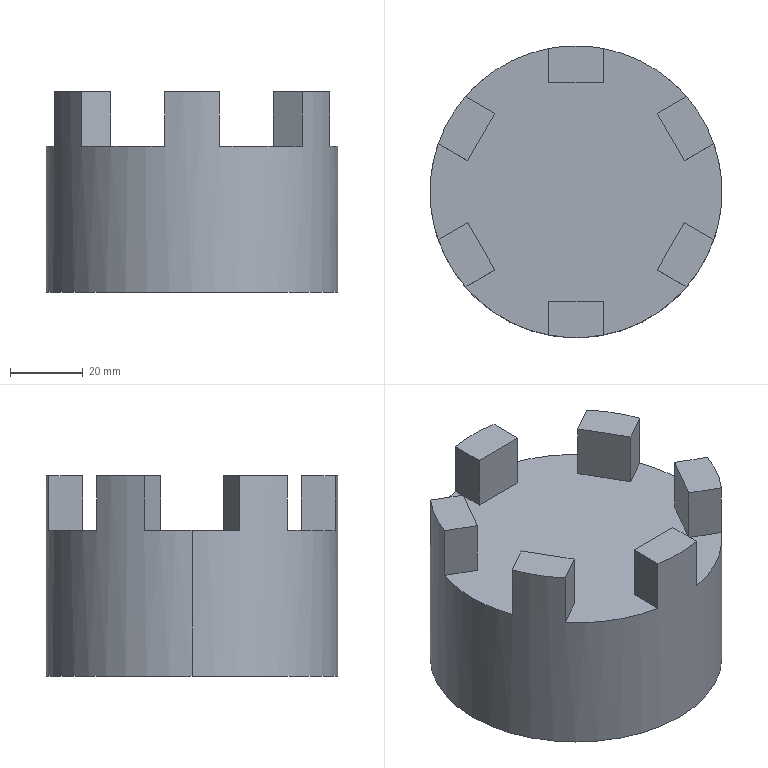Part | SolidWorks | features ICE 3, Extrusion 1 | 1 solid | 35 faces | box 80 x 80 x 55 mm | volume 187551 mm3 | plane 30 | cylinder 5 | commonest cylinder face diameters 33 x3 80 x2
STEP:
#1=CARTESIAN_POINT('',(40.,0.,40.));
#2=VERTEX_POINT('',#1);
#3=CARTESIAN_POINT('',(37.777,13.15,40.));
#4=VERTEX_POINT('',#3);
#5=CARTESIAN_POINT('',(0.,0.,40.));
#6=DIRECTION('',(0.,0.,1.));
#7=DIRECTION('',(1.,0.,0.));
#8=AXIS2_PLACEMENT_3D('',#5,#6,#7);
#9=CIRCLE('',#8,40.);
#10=EDGE_CURVE('',#2,#4,#9,.T.);
#11=ORIENTED_EDGE('',*,*,#10,.F.);
#12=CARTESIAN_POINT('',(40.,0.,0.));
#13=VERTEX_POINT('',#12);
#14=CARTESIAN_POINT('',(40.,0.,40.));
#15=DIRECTION('',(0.,0.,-1.));
#16=VECTOR('',#15,1000.);
#17=LINE('',#14,#16);
#18=EDGE_CURVE('',#2,#13,#17,.T.);
#19=ORIENTED_EDGE('',*,*,#18,.T.);
#20=CARTESIAN_POINT('',(-40.,0.,0.));
#21=VERTEX_POINT('',#20);
#22=CARTESIAN_POINT('',(0.,0.,0.));
#23=DIRECTION('',(0.,0.,1.));
#24=DIRECTION('',(1.,0.,0.));
#25=AXIS2_PLACEMENT_3D('',#22,#23,#24);
#26=CIRCLE('',#25,40.);
#27=EDGE_CURVE('',#13,#21,#26,.T.);
#28=ORIENTED_EDGE('',*,*,#27,.T.);
#29=CARTESIAN_POINT('',(-40.,0.,40.));
#30=VERTEX_POINT('',#29);
#31=CARTESIAN_POINT('',(-40.,0.,40.));
#32=DIRECTION('',(0.,0.,-1.));
#33=VECTOR('',#32,1000.);
#34=LINE('',#31,#33);
#35=EDGE_CURVE('',#30,#21,#34,.T.);
#36=ORIENTED_EDGE('',*,*,#35,.F.);
#37=CARTESIAN_POINT('',(-37.777,13.15,40.));
#38=VERTEX_POINT('',#37);
#39=CARTESIAN_POINT('',(0.,0.,40.));
#40=DIRECTION('',(0.,0.,1.));
#41=DIRECTION('',(1.,0.,0.));
#42=AXIS2_PLACEMENT_3D('',#39,#40,#41);
#43=CIRCLE('',#42,40.);
#44=EDGE_CURVE('',#38,#30,#43,.T.);
#45=ORIENTED_EDGE('',*,*,#44,.F.);
#46=CARTESIAN_POINT('',(-37.777,13.15,55.));
#47=VERTEX_POINT('',#46);
#48=CARTESIAN_POINT('',(-37.777,13.15,55.));
#49=DIRECTION('',(0.,0.,-1.));
#50=VECTOR('',#49,1000.);
#51=LINE('',#48,#50);
#52=EDGE_CURVE('',#47,#38,#51,.T.);
#53=ORIENTED_EDGE('',*,*,#52,.F.);
#54=CARTESIAN_POINT('',(-30.277,26.14,55.));
#55=VERTEX_POINT('',#54);
#56=CARTESIAN_POINT('',(0.,0.,55.));
#57=DIRECTION('',(0.,0.,1.));
#58=DIRECTION('',(1.,0.,0.));
#59=AXIS2_PLACEMENT_3D('',#56,#57,#58);
#60=CIRCLE('',#59,40.);
#61=EDGE_CURVE('',#55,#47,#60,.T.);
#62=ORIENTED_EDGE('',*,*,#61,.F.);
#63=CARTESIAN_POINT('',(-30.277,26.14,40.));
#64=VERTEX_POINT('',#63);
#65=CARTESIAN_POINT('',(-30.277,26.14,55.));
#66=DIRECTION('',(0.,0.,-1.));
#67=VECTOR('',#66,1000.);
#68=LINE('',#65,#67);
#69=EDGE_CURVE('',#55,#64,#68,.T.);
#70=ORIENTED_EDGE('',*,*,#69,.T.);
#71=CARTESIAN_POINT('',(-7.5,39.291,40.));
#72=VERTEX_POINT('',#71);
#73=CARTESIAN_POINT('',(0.,0.,40.));
#74=DIRECTION('',(0.,0.,1.));
#75=DIRECTION('',(1.,0.,0.));
#76=AXIS2_PLACEMENT_3D('',#73,#74,#75);
#77=CIRCLE('',#76,40.);
#78=EDGE_CURVE('',#72,#64,#77,.T.);
#79=ORIENTED_EDGE('',*,*,#78,.F.);
#80=CARTESIAN_POINT('',(-7.5,39.291,55.));
#81=VERTEX_POINT('',#80);
#82=CARTESIAN_POINT('',(-7.5,39.291,55.));
#83=DIRECTION('',(0.,0.,-1.));
#84=VECTOR('',#83,1000.);
#85=LINE('',#82,#84);
#86=EDGE_CURVE('',#81,#72,#85,.T.);
#87=ORIENTED_EDGE('',*,*,#86,.F.);
#88=CARTESIAN_POINT('',(7.5,39.291,55.));
#89=VERTEX_POINT('',#88);
#90=CARTESIAN_POINT('',(0.,0.,55.));
#91=DIRECTION('',(0.,0.,1.));
#92=DIRECTION('',(1.,0.,0.));
#93=AXIS2_PLACEMENT_3D('',#90,#91,#92);
#94=CIRCLE('',#93,40.);
#95=EDGE_CURVE('',#89,#81,#94,.T.);
#96=ORIENTED_EDGE('',*,*,#95,.F.);
#97=CARTESIAN_POINT('',(7.5,39.291,40.));
#98=VERTEX_POINT('',#97);
#99=CARTESIAN_POINT('',(7.5,39.291,55.));
#100=DIRECTION('',(0.,0.,-1.));
#101=VECTOR('',#100,1000.);
#102=LINE('',#99,#101);
#103=EDGE_CURVE('',#89,#98,#102,.T.);
#104=ORIENTED_EDGE('',*,*,#103,.T.);
#105=CARTESIAN_POINT('',(30.277,26.14,40.));
#106=VERTEX_POINT('',#105);
#107=CARTESIAN_POINT('',(0.,0.,40.));
#108=DIRECTION('',(0.,0.,1.));
#109=DIRECTION('',(1.,0.,0.));
#110=AXIS2_PLACEMENT_3D('',#107,#108,#109);
#111=CIRCLE('',#110,40.);
#112=EDGE_CURVE('',#106,#98,#111,.T.);
#113=ORIENTED_EDGE('',*,*,#112,.F.);
#114=CARTESIAN_POINT('',(30.277,26.14,55.));
#115=VERTEX_POINT('',#114);
#116=CARTESIAN_POINT('',(30.277,26.14,55.));
#117=DIRECTION('',(0.,0.,-1.));
#118=VECTOR('',#117,1000.);
#119=LINE('',#116,#118);
#120=EDGE_CURVE('',#115,#106,#119,.T.);
#121=ORIENTED_EDGE('',*,*,#120,.F.);
#122=CARTESIAN_POINT('',(37.777,13.15,55.));
#123=VERTEX_POINT('',#122);
#124=CARTESIAN_POINT('',(0.,0.,55.));
#125=DIRECTION('',(0.,0.,1.));
#126=DIRECTION('',(1.,0.,0.));
#127=AXIS2_PLACEMENT_3D('',#124,#125,#126);
#128=CIRCLE('',#127,40.);
#129=EDGE_CURVE('',#123,#115,#128,.T.);
#130=ORIENTED_EDGE('',*,*,#129,.F.);
#131=CARTESIAN_POINT('',(37.777,13.15,55.));
#132=DIRECTION('',(0.,0.,-1.));
#133=VECTOR('',#132,1000.);
#134=LINE('',#131,#133);
#135=EDGE_CURVE('',#123,#4,#134,.T.);
#136=ORIENTED_EDGE('',*,*,#135,.T.);
#137=EDGE_LOOP('',(#11,#19,#28,#36,#45,#53,#62,#70,#79,#87,#96,#104,#113,#121,#130,#136));
#138=FACE_OUTER_BOUND('',#137,.T.);
#139=CARTESIAN_POINT('',(0.,0.,40.));
#140=DIRECTION('',(0.,0.,-1.));
#141=DIRECTION('',(-1.,0.,0.));
#142=AXIS2_PLACEMENT_3D('',#139,#140,#141);
#143=CYLINDRICAL_SURFACE('',#142,40.);
#144=ADVANCED_FACE('',(#138),#143,.T.);
#145=CARTESIAN_POINT('',(-16.5,0.,30.));
#146=VERTEX_POINT('',#145);
#147=CARTESIAN_POINT('',(16.5,0.,30.));
#148=VERTEX_POINT('',#147);
#149=CARTESIAN_POINT('',(0.,0.,30.));
#150=DIRECTION('',(0.,0.,1.));
#151=DIRECTION('',(1.,0.,0.));
#152=AXIS2_PLACEMENT_3D('',#149,#150,#151);
#153=CIRCLE('',#152,16.5);
#154=EDGE_CURVE('',#146,#148,#153,.T.);
#155=ORIENTED_EDGE('',*,*,#154,.T.);
#156=CARTESIAN_POINT('',(16.5,0.,0.));
#157=VERTEX_POINT('',#156);
#158=CARTESIAN_POINT('',(16.5,0.,30.));
#159=DIRECTION('',(0.,0.,-1.));
#160=VECTOR('',#159,1000.);
#161=LINE('',#158,#160);
#162=EDGE_CURVE('',#148,#157,#161,.T.);
#163=ORIENTED_EDGE('',*,*,#162,.T.);
#164=CARTESIAN_POINT('',(-16.5,0.,0.));
#165=VERTEX_POINT('',#164);
#166=CARTESIAN_POINT('',(0.,0.,0.));
#167=DIRECTION('',(0.,0.,1.));
#168=DIRECTION('',(1.,0.,0.));
#169=AXIS2_PLACEMENT_3D('',#166,#167,#168);
#170=CIRCLE('',#169,16.5);
#171=EDGE_CURVE('',#165,#157,#170,.T.);
#172=ORIENTED_EDGE('',*,*,#171,.F.);
#173=CARTESIAN_POINT('',(-16.5,0.,30.));
#174=DIRECTION('',(0.,0.,-1.));
#175=VECTOR('',#174,1000.);
#176=LINE('',#173,#175);
#177=EDGE_CURVE('',#146,#165,#176,.T.);
#178=ORIENTED_EDGE('',*,*,#177,.F.);
#179=EDGE_LOOP('',(#155,#163,#172,#178));
#180=FACE_OUTER_BOUND('',#179,.T.);
#181=CARTESIAN_POINT('',(0.,0.,30.));
#182=DIRECTION('',(0.,0.,-1.));
#183=DIRECTION('',(-1.,0.,0.));
#184=AXIS2_PLACEMENT_3D('',#181,#182,#183);
#185=CYLINDRICAL_SURFACE('',#184,16.5);
#186=ADVANCED_FACE('',(#180),#185,.F.);
#187=CARTESIAN_POINT('',(-6.,15.37,30.));
#188=VERTEX_POINT('',#187);
#189=CARTESIAN_POINT('',(0.,0.,30.));
#190=DIRECTION('',(0.,0.,1.));
#191=DIRECTION('',(1.,0.,0.));
#192=AXIS2_PLACEMENT_3D('',#189,#190,#191);
#193=CIRCLE('',#192,16.5);
#194=EDGE_CURVE('',#188,#146,#193,.T.);
#195=ORIENTED_EDGE('',*,*,#194,.T.);
#196=ORIENTED_EDGE('',*,*,#177,.T.);
#197=CARTESIAN_POINT('',(-6.,15.37,0.));
#198=VERTEX_POINT('',#197);
#199=CARTESIAN_POINT('',(0.,0.,0.));
#200=DIRECTION('',(0.,0.,1.));
#201=DIRECTION('',(1.,0.,0.));
#202=AXIS2_PLACEMENT_3D('',#199,#200,#201);
#203=CIRCLE('',#202,16.5);
#204=EDGE_CURVE('',#198,#165,#203,.T.);
#205=ORIENTED_EDGE('',*,*,#204,.F.);
#206=CARTESIAN_POINT('',(-6.,15.37,30.));
#207=DIRECTION('',(0.,0.,1.));
#208=VECTOR('',#207,1000.);
#209=LINE('',#206,#208);
#210=EDGE_CURVE('',#198,#188,#209,.T.);
#211=ORIENTED_EDGE('',*,*,#210,.T.);
#212=EDGE_LOOP('',(#195,#196,#205,#211));
#213=FACE_OUTER_BOUND('',#212,.T.);
#214=CARTESIAN_POINT('',(0.,0.,30.));
#215=DIRECTION('',(0.,0.,-1.));
#216=DIRECTION('',(-1.,0.,0.));
#217=AXIS2_PLACEMENT_3D('',#214,#215,#216);
#218=CYLINDRICAL_SURFACE('',#217,16.5);
#219=ADVANCED_FACE('',(#213),#218,.F.);
#220=CARTESIAN_POINT('',(0.,0.,0.));
#221=DIRECTION('',(0.,0.,1.));
#222=DIRECTION('',(1.,0.,0.));
#223=AXIS2_PLACEMENT_3D('',#220,#221,#222);
#224=CIRCLE('',#223,40.);
#225=EDGE_CURVE('',#21,#13,#224,.T.);
#226=ORIENTED_EDGE('',*,*,#225,.F.);
#227=ORIENTED_EDGE('',*,*,#27,.F.);
#228=EDGE_LOOP('',(#226,#227));
#229=FACE_OUTER_BOUND('',#228,.T.);
#230=CARTESIAN_POINT('',(-6.,19.,0.));
#231=VERTEX_POINT('',#230);
#232=CARTESIAN_POINT('',(-6.,19.,0.));
#233=DIRECTION('',(0.,-1.,0.));
#234=VECTOR('',#233,1000.);
#235=LINE('',#232,#234);
#236=EDGE_CURVE('',#231,#198,#235,.T.);
#237=ORIENTED_EDGE('',*,*,#236,.T.);
#238=ORIENTED_EDGE('',*,*,#204,.T.);
#239=ORIENTED_EDGE('',*,*,#171,.T.);
#240=CARTESIAN_POINT('',(6.,15.37,0.));
#241=VERTEX_POINT('',#240);
#242=CARTESIAN_POINT('',(0.,0.,0.));
#243=DIRECTION('',(0.,0.,1.));
#244=DIRECTION('',(1.,0.,0.));
#245=AXIS2_PLACEMENT_3D('',#242,#243,#244);
#246=CIRCLE('',#245,16.5);
#247=EDGE_CURVE('',#157,#241,#246,.T.);
#248=ORIENTED_EDGE('',*,*,#247,.T.);
#249=CARTESIAN_POINT('',(6.,19.,0.));
#250=VERTEX_POINT('',#249);
#251=CARTESIAN_POINT('',(6.,19.,0.));
#252=DIRECTION('',(0.,-1.,0.));
#253=VECTOR('',#252,1000.);
#254=LINE('',#251,#253);
#255=EDGE_CURVE('',#250,#241,#254,.T.);
#256=ORIENTED_EDGE('',*,*,#255,.F.);
#257=CARTESIAN_POINT('',(6.,19.,0.));
#258=DIRECTION('',(-1.,0.,0.));
#259=VECTOR('',#258,1000.);
#260=LINE('',#257,#259);
#261=EDGE_CURVE('',#250,#231,#260,.T.);
#262=ORIENTED_EDGE('',*,*,#261,.T.);
#263=EDGE_LOOP('',(#237,#238,#239,#248,#256,#262));
#264=FACE_BOUND('',#263,.T.);
#265=CARTESIAN_POINT('',(0.,0.,0.));
#266=DIRECTION('',(0.,0.,1.));
#267=DIRECTION('',(1.,0.,0.));
#268=AXIS2_PLACEMENT_3D('',#265,#266,#267);
#269=PLANE('',#268);
#270=ADVANCED_FACE('',(#229,#264),#269,.F.);
#271=ORIENTED_EDGE('',*,*,#162,.F.);
#272=CARTESIAN_POINT('',(6.,15.37,30.));
#273=VERTEX_POINT('',#272);
#274=CARTESIAN_POINT('',(0.,0.,30.));
#275=DIRECTION('',(0.,0.,1.));
#276=DIRECTION('',(1.,0.,0.));
#277=AXIS2_PLACEMENT_3D('',#274,#275,#276);
#278=CIRCLE('',#277,16.5);
#279=EDGE_CURVE('',#148,#273,#278,.T.);
#280=ORIENTED_EDGE('',*,*,#279,.T.);
#281=CARTESIAN_POINT('',(6.,15.37,30.));
#282=DIRECTION('',(0.,0.,1.));
#283=VECTOR('',#282,1000.);
#284=LINE('',#281,#283);
#285=EDGE_CURVE('',#241,#273,#284,.T.);
#286=ORIENTED_EDGE('',*,*,#285,.F.);
#287=ORIENTED_EDGE('',*,*,#247,.F.);
#288=EDGE_LOOP('',(#271,#280,#286,#287));
#289=FACE_OUTER_BOUND('',#288,.T.);
#290=CARTESIAN_POINT('',(0.,0.,30.));
#291=DIRECTION('',(0.,0.,-1.));
#292=DIRECTION('',(-1.,0.,0.));
#293=AXIS2_PLACEMENT_3D('',#290,#291,#292);
#294=CYLINDRICAL_SURFACE('',#293,16.5);
#295=ADVANCED_FACE('',(#289),#294,.F.);
#296=ORIENTED_EDGE('',*,*,#18,.F.);
#297=CARTESIAN_POINT('',(37.777,-13.15,40.));
#298=VERTEX_POINT('',#297);
#299=CARTESIAN_POINT('',(0.,0.,40.));
#300=DIRECTION('',(0.,0.,1.));
#301=DIRECTION('',(1.,0.,0.));
#302=AXIS2_PLACEMENT_3D('',#299,#300,#301);
#303=CIRCLE('',#302,40.);
#304=EDGE_CURVE('',#298,#2,#303,.T.);
#305=ORIENTED_EDGE('',*,*,#304,.F.);
#306=CARTESIAN_POINT('',(37.777,-13.15,55.));
#307=VERTEX_POINT('',#306);
#308=CARTESIAN_POINT('',(37.777,-13.15,55.));
#309=DIRECTION('',(0.,0.,-1.));
#310=VECTOR('',#309,1000.);
#311=LINE('',#308,#310);
#312=EDGE_CURVE('',#307,#298,#311,.T.);
#313=ORIENTED_EDGE('',*,*,#312,.F.);
#314=CARTESIAN_POINT('',(30.277,-26.14,55.));
#315=VERTEX_POINT('',#314);
#316=CARTESIAN_POINT('',(0.,0.,55.));
#317=DIRECTION('',(0.,0.,1.));
#318=DIRECTION('',(1.,0.,0.));
#319=AXIS2_PLACEMENT_3D('',#316,#317,#318);
#320=CIRCLE('',#319,40.);
#321=EDGE_CURVE('',#315,#307,#320,.T.);
#322=ORIENTED_EDGE('',*,*,#321,.F.);
#323=CARTESIAN_POINT('',(30.277,-26.14,40.));
#324=VERTEX_POINT('',#323);
#325=CARTESIAN_POINT('',(30.277,-26.14,55.));
#326=DIRECTION('',(0.,0.,-1.));
#327=VECTOR('',#326,1000.);
#328=LINE('',#325,#327);
#329=EDGE_CURVE('',#315,#324,#328,.T.);
#330=ORIENTED_EDGE('',*,*,#329,.T.);
#331=CARTESIAN_POINT('',(7.5,-39.291,40.));
#332=VERTEX_POINT('',#331);
#333=CARTESIAN_POINT('',(0.,0.,40.));
#334=DIRECTION('',(0.,0.,1.));
#335=DIRECTION('',(1.,0.,0.));
#336=AXIS2_PLACEMENT_3D('',#333,#334,#335);
#337=CIRCLE('',#336,40.);
#338=EDGE_CURVE('',#332,#324,#337,.T.);
#339=ORIENTED_EDGE('',*,*,#338,.F.);
#340=CARTESIAN_POINT('',(7.5,-39.291,55.));
#341=VERTEX_POINT('',#340);
#342=CARTESIAN_POINT('',(7.5,-39.291,55.));
#343=DIRECTION('',(0.,0.,-1.));
#344=VECTOR('',#343,1000.);
#345=LINE('',#342,#344);
#346=EDGE_CURVE('',#341,#332,#345,.T.);
#347=ORIENTED_EDGE('',*,*,#346,.F.);
#348=CARTESIAN_POINT('',(-7.5,-39.291,55.));
#349=VERTEX_POINT('',#348);
#350=CARTESIAN_POINT('',(0.,0.,55.));
#351=DIRECTION('',(0.,0.,1.));
#352=DIRECTION('',(1.,0.,0.));
#353=AXIS2_PLACEMENT_3D('',#350,#351,#352);
#354=CIRCLE('',#353,40.);
#355=EDGE_CURVE('',#349,#341,#354,.T.);
#356=ORIENTED_EDGE('',*,*,#355,.F.);
#357=CARTESIAN_POINT('',(-7.5,-39.291,40.));
#358=VERTEX_POINT('',#357);
#359=CARTESIAN_POINT('',(-7.5,-39.291,55.));
#360=DIRECTION('',(0.,0.,-1.));
#361=VECTOR('',#360,1000.);
#362=LINE('',#359,#361);
#363=EDGE_CURVE('',#349,#358,#362,.T.);
#364=ORIENTED_EDGE('',*,*,#363,.T.);
#365=CARTESIAN_POINT('',(-30.277,-26.14,40.));
#366=VERTEX_POINT('',#365);
#367=CARTESIAN_POINT('',(0.,0.,40.));
#368=DIRECTION('',(0.,0.,1.));
#369=DIRECTION('',(1.,0.,0.));
#370=AXIS2_PLACEMENT_3D('',#367,#368,#369);
#371=CIRCLE('',#370,40.);
#372=EDGE_CURVE('',#366,#358,#371,.T.);
#373=ORIENTED_EDGE('',*,*,#372,.F.);
#374=CARTESIAN_POINT('',(-30.277,-26.14,55.));
#375=VERTEX_POINT('',#374);
#376=CARTESIAN_POINT('',(-30.277,-26.14,55.));
#377=DIRECTION('',(0.,0.,-1.));
#378=VECTOR('',#377,1000.);
#379=LINE('',#376,#378);
#380=EDGE_CURVE('',#375,#366,#379,.T.);
#381=ORIENTED_EDGE('',*,*,#380,.F.);
#382=CARTESIAN_POINT('',(-37.777,-13.15,55.));
#383=VERTEX_POINT('',#382);
#384=CARTESIAN_POINT('',(0.,0.,55.));
#385=DIRECTION('',(0.,0.,1.));
#386=DIRECTION('',(1.,0.,0.));
#387=AXIS2_PLACEMENT_3D('',#384,#385,#386);
#388=CIRCLE('',#387,40.);
#389=EDGE_CURVE('',#383,#375,#388,.T.);
#390=ORIENTED_EDGE('',*,*,#389,.F.);
#391=CARTESIAN_POINT('',(-37.777,-13.15,40.));
#392=VERTEX_POINT('',#391);
#393=CARTESIAN_POINT('',(-37.777,-13.15,55.));
#394=DIRECTION('',(0.,0.,-1.));
#395=VECTOR('',#394,1000.);
#396=LINE('',#393,#395);
#397=EDGE_CURVE('',#383,#392,#396,.T.);
#398=ORIENTED_EDGE('',*,*,#397,.T.);
#399=CARTESIAN_POINT('',(0.,0.,40.));
#400=DIRECTION('',(0.,0.,1.));
#401=DIRECTION('',(1.,0.,0.));
#402=AXIS2_PLACEMENT_3D('',#399,#400,#401);
#403=CIRCLE('',#402,40.);
#404=EDGE_CURVE('',#30,#392,#403,.T.);
#405=ORIENTED_EDGE('',*,*,#404,.F.);
#406=ORIENTED_EDGE('',*,*,#35,.T.);
#407=ORIENTED_EDGE('',*,*,#225,.T.);
#408=EDGE_LOOP('',(#296,#305,#313,#322,#330,#339,#347,#356,#364,#373,#381,#390,#398,#405,#406,#407));
#409=FACE_OUTER_BOUND('',#408,.T.);
#410=CARTESIAN_POINT('',(0.,0.,40.));
#411=DIRECTION('',(0.,0.,-1.));
#412=DIRECTION('',(-1.,0.,0.));
#413=AXIS2_PLACEMENT_3D('',#410,#411,#412);
#414=CYLINDRICAL_SURFACE('',#413,40.);
#415=ADVANCED_FACE('',(#409),#414,.T.);
#416=CARTESIAN_POINT('',(7.5,30.,40.));
#417=VERTEX_POINT('',#416);
#418=CARTESIAN_POINT('',(7.5,39.291,40.));
#419=DIRECTION('',(0.,1.,0.));
#420=VECTOR('',#419,1000.);
#421=LINE('',#418,#420);
#422=EDGE_CURVE('',#417,#98,#421,.T.);
#423=ORIENTED_EDGE('',*,*,#422,.F.);
#424=CARTESIAN_POINT('',(-7.5,30.,40.));
#425=VERTEX_POINT('',#424);
#426=CARTESIAN_POINT('',(-7.5,30.,40.));
#427=DIRECTION('',(1.,0.,0.));
#428=VECTOR('',#427,1000.);
#429=LINE('',#426,#428);
#430=EDGE_CURVE('',#425,#417,#429,.T.);
#431=ORIENTED_EDGE('',*,*,#430,.F.);
#432=CARTESIAN_POINT('',(-7.5,39.291,40.));
#433=DIRECTION('',(0.,-1.,0.));
#434=VECTOR('',#433,1000.);
#435=LINE('',#432,#434);
#436=EDGE_CURVE('',#72,#425,#435,.T.);
#437=ORIENTED_EDGE('',*,*,#436,.F.);
#438=ORIENTED_EDGE('',*,*,#78,.T.);
#439=CARTESIAN_POINT('',(-22.231,21.495,40.));
#440=VERTEX_POINT('',#439);
#441=CARTESIAN_POINT('',(-30.277,26.14,40.));
#442=DIRECTION('',(-0.866,0.5,0.));
#443=VECTOR('',#442,1000.);
#444=LINE('',#441,#443);
#445=EDGE_CURVE('',#440,#64,#444,.T.);
#446=ORIENTED_EDGE('',*,*,#445,.F.);
#447=CARTESIAN_POINT('',(-29.731,8.505,40.));
#448=VERTEX_POINT('',#447);
#449=CARTESIAN_POINT('',(-29.731,8.505,40.));
#450=DIRECTION('',(0.5,0.866,0.));
#451=VECTOR('',#450,1000.);
#452=LINE('',#449,#451);
#453=EDGE_CURVE('',#448,#440,#452,.T.);
#454=ORIENTED_EDGE('',*,*,#453,.F.);
#455=CARTESIAN_POINT('',(-37.777,13.15,40.));
#456=DIRECTION('',(0.866,-0.5,0.));
#457=VECTOR('',#456,1000.);
#458=LINE('',#455,#457);
#459=EDGE_CURVE('',#38,#448,#458,.T.);
#460=ORIENTED_EDGE('',*,*,#459,.F.);
#461=ORIENTED_EDGE('',*,*,#44,.T.);
#462=ORIENTED_EDGE('',*,*,#404,.T.);
#463=CARTESIAN_POINT('',(-29.731,-8.505,40.));
#464=VERTEX_POINT('',#463);
#465=CARTESIAN_POINT('',(-37.777,-13.15,40.));
#466=DIRECTION('',(-0.866,-0.5,0.));
#467=VECTOR('',#466,1000.);
#468=LINE('',#465,#467);
#469=EDGE_CURVE('',#464,#392,#468,.T.);
#470=ORIENTED_EDGE('',*,*,#469,.F.);
#471=CARTESIAN_POINT('',(-22.231,-21.495,40.));
#472=VERTEX_POINT('',#471);
#473=CARTESIAN_POINT('',(-22.231,-21.495,40.));
#474=DIRECTION('',(-0.5,0.866,0.));
#475=VECTOR('',#474,1000.);
#476=LINE('',#473,#475);
#477=EDGE_CURVE('',#472,#464,#476,.T.);
#478=ORIENTED_EDGE('',*,*,#477,.F.);
#479=CARTESIAN_POINT('',(-30.277,-26.14,40.));
#480=DIRECTION('',(0.866,0.5,0.));
#481=VECTOR('',#480,1000.);
#482=LINE('',#479,#481);
#483=EDGE_CURVE('',#366,#472,#482,.T.);
#484=ORIENTED_EDGE('',*,*,#483,.F.);
#485=ORIENTED_EDGE('',*,*,#372,.T.);
#486=CARTESIAN_POINT('',(-7.5,-30.,40.));
#487=VERTEX_POINT('',#486);
#488=CARTESIAN_POINT('',(-7.5,-39.291,40.));
#489=DIRECTION('',(0.,-1.,0.));
#490=VECTOR('',#489,1000.);
#491=LINE('',#488,#490);
#492=EDGE_CURVE('',#487,#358,#491,.T.);
#493=ORIENTED_EDGE('',*,*,#492,.F.);
#494=CARTESIAN_POINT('',(7.5,-30.,40.));
#495=VERTEX_POINT('',#494);
#496=CARTESIAN_POINT('',(7.5,-30.,40.));
#497=DIRECTION('',(-1.,0.,0.));
#498=VECTOR('',#497,1000.);
#499=LINE('',#496,#498);
#500=EDGE_CURVE('',#495,#487,#499,.T.);
#501=ORIENTED_EDGE('',*,*,#500,.F.);
#502=CARTESIAN_POINT('',(7.5,-39.291,40.));
#503=DIRECTION('',(0.,1.,0.));
#504=VECTOR('',#503,1000.);
#505=LINE('',#502,#504);
#506=EDGE_CURVE('',#332,#495,#505,.T.);
#507=ORIENTED_EDGE('',*,*,#506,.F.);
#508=ORIENTED_EDGE('',*,*,#338,.T.);
#509=CARTESIAN_POINT('',(22.231,-21.495,40.));
#510=VERTEX_POINT('',#509);
#511=CARTESIAN_POINT('',(30.277,-26.14,40.));
#512=DIRECTION('',(0.866,-0.5,0.));
#513=VECTOR('',#512,1000.);
#514=LINE('',#511,#513);
#515=EDGE_CURVE('',#510,#324,#514,.T.);
#516=ORIENTED_EDGE('',*,*,#515,.F.);
#517=CARTESIAN_POINT('',(29.731,-8.505,40.));
#518=VERTEX_POINT('',#517);
#519=CARTESIAN_POINT('',(29.731,-8.505,40.));
#520=DIRECTION('',(-0.5,-0.866,0.));
#521=VECTOR('',#520,1000.);
#522=LINE('',#519,#521);
#523=EDGE_CURVE('',#518,#510,#522,.T.);
#524=ORIENTED_EDGE('',*,*,#523,.F.);
#525=CARTESIAN_POINT('',(37.777,-13.15,40.));
#526=DIRECTION('',(-0.866,0.5,0.));
#527=VECTOR('',#526,1000.);
#528=LINE('',#525,#527);
#529=EDGE_CURVE('',#298,#518,#528,.T.);
#530=ORIENTED_EDGE('',*,*,#529,.F.);
#531=ORIENTED_EDGE('',*,*,#304,.T.);
#532=ORIENTED_EDGE('',*,*,#10,.T.);
#533=CARTESIAN_POINT('',(29.731,8.505,40.));
#534=VERTEX_POINT('',#533);
#535=CARTESIAN_POINT('',(37.777,13.15,40.));
#536=DIRECTION('',(0.866,0.5,0.));
#537=VECTOR('',#536,1000.);
#538=LINE('',#535,#537);
#539=EDGE_CURVE('',#534,#4,#538,.T.);
#540=ORIENTED_EDGE('',*,*,#539,.F.);
#541=CARTESIAN_POINT('',(22.231,21.495,40.));
#542=VERTEX_POINT('',#541);
#543=CARTESIAN_POINT('',(22.231,21.495,40.));
#544=DIRECTION('',(0.5,-0.866,0.));
#545=VECTOR('',#544,1000.);
#546=LINE('',#543,#545);
#547=EDGE_CURVE('',#542,#534,#546,.T.);
#548=ORIENTED_EDGE('',*,*,#547,.F.);
#549=CARTESIAN_POINT('',(30.277,26.14,40.));
#550=DIRECTION('',(-0.866,-0.5,0.));
#551=VECTOR('',#550,1000.);
#552=LINE('',#549,#551);
#553=EDGE_CURVE('',#106,#542,#552,.T.);
#554=ORIENTED_EDGE('',*,*,#553,.F.);
#555=ORIENTED_EDGE('',*,*,#112,.T.);
#556=EDGE_LOOP('',(#423,#431,#437,#438,#446,#454,#460,#461,#462,#470,#478,#484,#485,#493,#501,#507,#508,#516,#524,#530,#531,#532,#540,#548,#554,#555));
#557=FACE_OUTER_BOUND('',#556,.T.);
#558=CARTESIAN_POINT('',(0.,0.,40.));
#559=DIRECTION('',(0.,0.,1.));
#560=DIRECTION('',(1.,0.,0.));
#561=AXIS2_PLACEMENT_3D('',#558,#559,#560);
#562=PLANE('',#561);
#563=ADVANCED_FACE('',(#557),#562,.T.);
#564=ORIENTED_EDGE('',*,*,#194,.F.);
#565=CARTESIAN_POINT('',(-6.,19.,30.));
#566=VERTEX_POINT('',#565);
#567=CARTESIAN_POINT('',(-6.,19.,30.));
#568=DIRECTION('',(0.,-1.,0.));
#569=VECTOR('',#568,1000.);
#570=LINE('',#567,#569);
#571=EDGE_CURVE('',#566,#188,#570,.T.);
#572=ORIENTED_EDGE('',*,*,#571,.F.);
#573=CARTESIAN_POINT('',(6.,19.,30.));
#574=VERTEX_POINT('',#573);
#575=CARTESIAN_POINT('',(6.,19.,30.));
#576=DIRECTION('',(-1.,0.,0.));
#577=VECTOR('',#576,1000.);
#578=LINE('',#575,#577);
#579=EDGE_CURVE('',#574,#566,#578,.T.);
#580=ORIENTED_EDGE('',*,*,#579,.F.);
#581=CARTESIAN_POINT('',(6.,19.,30.));
#582=DIRECTION('',(0.,-1.,0.));
#583=VECTOR('',#582,1000.);
#584=LINE('',#581,#583);
#585=EDGE_CURVE('',#574,#273,#584,.T.);
#586=ORIENTED_EDGE('',*,*,#585,.T.);
#587=ORIENTED_EDGE('',*,*,#279,.F.);
#588=ORIENTED_EDGE('',*,*,#154,.F.);
#589=EDGE_LOOP('',(#564,#572,#580,#586,#587,#588));
#590=FACE_OUTER_BOUND('',#589,.T.);
#591=CARTESIAN_POINT('',(0.,0.,30.));
#592=DIRECTION('',(0.,0.,1.));
#593=DIRECTION('',(1.,0.,0.));
#594=AXIS2_PLACEMENT_3D('',#591,#592,#593);
#595=PLANE('',#594);
#596=ADVANCED_FACE('',(#590),#595,.F.);
#597=ORIENTED_EDGE('',*,*,#539,.T.);
#598=ORIENTED_EDGE('',*,*,#135,.F.);
#599=CARTESIAN_POINT('',(29.731,8.505,55.));
#600=VERTEX_POINT('',#599);
#601=CARTESIAN_POINT('',(37.777,13.15,55.));
#602=DIRECTION('',(0.866,0.5,0.));
#603=VECTOR('',#602,1000.);
#604=LINE('',#601,#603);
#605=EDGE_CURVE('',#600,#123,#604,.T.);
#606=ORIENTED_EDGE('',*,*,#605,.F.);
#607=CARTESIAN_POINT('',(29.731,8.505,55.));
#608=DIRECTION('',(0.,0.,-1.));
#609=VECTOR('',#608,1000.);
#610=LINE('',#607,#609);
#611=EDGE_CURVE('',#600,#534,#610,.T.);
#612=ORIENTED_EDGE('',*,*,#611,.T.);
#613=EDGE_LOOP('',(#597,#598,#606,#612));
#614=FACE_OUTER_BOUND('',#613,.T.);
#615=CARTESIAN_POINT('',(37.777,13.15,55.));
#616=DIRECTION('',(-0.5,0.866,0.));
#617=DIRECTION('',(-0.866,-0.5,0.));
#618=AXIS2_PLACEMENT_3D('',#615,#616,#617);
#619=PLANE('',#618);
#620=ADVANCED_FACE('',(#614),#619,.F.);
#621=ORIENTED_EDGE('',*,*,#553,.T.);
#622=CARTESIAN_POINT('',(22.231,21.495,55.));
#623=VERTEX_POINT('',#622);
#624=CARTESIAN_POINT('',(22.231,21.495,55.));
#625=DIRECTION('',(0.,0.,-1.));
#626=VECTOR('',#625,1000.);
#627=LINE('',#624,#626);
#628=EDGE_CURVE('',#623,#542,#627,.T.);
#629=ORIENTED_EDGE('',*,*,#628,.F.);
#630=CARTESIAN_POINT('',(30.277,26.14,55.));
#631=DIRECTION('',(-0.866,-0.5,0.));
#632=VECTOR('',#631,1000.);
#633=LINE('',#630,#632);
#634=EDGE_CURVE('',#115,#623,#633,.T.);
#635=ORIENTED_EDGE('',*,*,#634,.F.);
#636=ORIENTED_EDGE('',*,*,#120,.T.);
#637=EDGE_LOOP('',(#621,#629,#635,#636));
#638=FACE_OUTER_BOUND('',#637,.T.);
#639=CARTESIAN_POINT('',(30.277,26.14,55.));
#640=DIRECTION('',(0.5,-0.866,0.));
#641=DIRECTION('',(0.866,0.5,0.));
#642=AXIS2_PLACEMENT_3D('',#639,#640,#641);
#643=PLANE('',#642);
#644=ADVANCED_FACE('',(#638),#643,.F.);
#645=ORIENTED_EDGE('',*,*,#547,.T.);
#646=ORIENTED_EDGE('',*,*,#611,.F.);
#647=CARTESIAN_POINT('',(22.231,21.495,55.));
#648=DIRECTION('',(0.5,-0.866,0.));
#649=VECTOR('',#648,1000.);
#650=LINE('',#647,#649);
#651=EDGE_CURVE('',#623,#600,#650,.T.);
#652=ORIENTED_EDGE('',*,*,#651,.F.);
#653=ORIENTED_EDGE('',*,*,#628,.T.);
#654=EDGE_LOOP('',(#645,#646,#652,#653));
#655=FACE_OUTER_BOUND('',#654,.T.);
#656=CARTESIAN_POINT('',(22.231,21.495,55.));
#657=DIRECTION('',(0.866,0.5,0.));
#658=DIRECTION('',(-0.5,0.866,0.));
#659=AXIS2_PLACEMENT_3D('',#656,#657,#658);
#660=PLANE('',#659);
#661=ADVANCED_FACE('',(#655),#660,.F.);
#662=ORIENTED_EDGE('',*,*,#605,.T.);
#663=ORIENTED_EDGE('',*,*,#129,.T.);
#664=ORIENTED_EDGE('',*,*,#634,.T.);
#665=ORIENTED_EDGE('',*,*,#651,.T.);
#666=EDGE_LOOP('',(#662,#663,#664,#665));
#667=FACE_OUTER_BOUND('',#666,.T.);
#668=CARTESIAN_POINT('',(0.,0.,55.));
#669=DIRECTION('',(0.,0.,1.));
#670=DIRECTION('',(1.,0.,0.));
#671=AXIS2_PLACEMENT_3D('',#668,#669,#670);
#672=PLANE('',#671);
#673=ADVANCED_FACE('',(#667),#672,.T.);
#674=ORIENTED_EDGE('',*,*,#515,.T.);
#675=ORIENTED_EDGE('',*,*,#329,.F.);
#676=CARTESIAN_POINT('',(22.231,-21.495,55.));
#677=VERTEX_POINT('',#676);
#678=CARTESIAN_POINT('',(30.277,-26.14,55.));
#679=DIRECTION('',(0.866,-0.5,0.));
#680=VECTOR('',#679,1000.);
#681=LINE('',#678,#680);
#682=EDGE_CURVE('',#677,#315,#681,.T.);
#683=ORIENTED_EDGE('',*,*,#682,.F.);
#684=CARTESIAN_POINT('',(22.231,-21.495,55.));
#685=DIRECTION('',(0.,0.,-1.));
#686=VECTOR('',#685,1000.);
#687=LINE('',#684,#686);
#688=EDGE_CURVE('',#677,#510,#687,.T.);
#689=ORIENTED_EDGE('',*,*,#688,.T.);
#690=EDGE_LOOP('',(#674,#675,#683,#689));
#691=FACE_OUTER_BOUND('',#690,.T.);
#692=CARTESIAN_POINT('',(30.277,-26.14,55.));
#693=DIRECTION('',(0.5,0.866,0.));
#694=DIRECTION('',(-0.866,0.5,0.));
#695=AXIS2_PLACEMENT_3D('',#692,#693,#694);
#696=PLANE('',#695);
#697=ADVANCED_FACE('',(#691),#696,.F.);
#698=ORIENTED_EDGE('',*,*,#529,.T.);
#699=CARTESIAN_POINT('',(29.731,-8.505,55.));
#700=VERTEX_POINT('',#699);
#701=CARTESIAN_POINT('',(29.731,-8.505,55.));
#702=DIRECTION('',(0.,0.,-1.));
#703=VECTOR('',#702,1000.);
#704=LINE('',#701,#703);
#705=EDGE_CURVE('',#700,#518,#704,.T.);
#706=ORIENTED_EDGE('',*,*,#705,.F.);
#707=CARTESIAN_POINT('',(37.777,-13.15,55.));
#708=DIRECTION('',(-0.866,0.5,0.));
#709=VECTOR('',#708,1000.);
#710=LINE('',#707,#709);
#711=EDGE_CURVE('',#307,#700,#710,.T.);
#712=ORIENTED_EDGE('',*,*,#711,.F.);
#713=ORIENTED_EDGE('',*,*,#312,.T.);
#714=EDGE_LOOP('',(#698,#706,#712,#713));
#715=FACE_OUTER_BOUND('',#714,.T.);
#716=CARTESIAN_POINT('',(37.777,-13.15,55.));
#717=DIRECTION('',(-0.5,-0.866,0.));
#718=DIRECTION('',(0.866,-0.5,0.));
#719=AXIS2_PLACEMENT_3D('',#716,#717,#718);
#720=PLANE('',#719);
#721=ADVANCED_FACE('',(#715),#720,.F.);
#722=ORIENTED_EDGE('',*,*,#523,.T.);
#723=ORIENTED_EDGE('',*,*,#688,.F.);
#724=CARTESIAN_POINT('',(29.731,-8.505,55.));
#725=DIRECTION('',(-0.5,-0.866,0.));
#726=VECTOR('',#725,1000.);
#727=LINE('',#724,#726);
#728=EDGE_CURVE('',#700,#677,#727,.T.);
#729=ORIENTED_EDGE('',*,*,#728,.F.);
#730=ORIENTED_EDGE('',*,*,#705,.T.);
#731=EDGE_LOOP('',(#722,#723,#729,#730));
#732=FACE_OUTER_BOUND('',#731,.T.);
#733=CARTESIAN_POINT('',(29.731,-8.505,55.));
#734=DIRECTION('',(0.866,-0.5,0.));
#735=DIRECTION('',(0.5,0.866,0.));
#736=AXIS2_PLACEMENT_3D('',#733,#734,#735);
#737=PLANE('',#736);
#738=ADVANCED_FACE('',(#732),#737,.F.);
#739=ORIENTED_EDGE('',*,*,#682,.T.);
#740=ORIENTED_EDGE('',*,*,#321,.T.);
#741=ORIENTED_EDGE('',*,*,#711,.T.);
#742=ORIENTED_EDGE('',*,*,#728,.T.);
#743=EDGE_LOOP('',(#739,#740,#741,#742));
#744=FACE_OUTER_BOUND('',#743,.T.);
#745=CARTESIAN_POINT('',(0.,0.,55.));
#746=DIRECTION('',(0.,0.,1.));
#747=DIRECTION('',(1.,0.,0.));
#748=AXIS2_PLACEMENT_3D('',#745,#746,#747);
#749=PLANE('',#748);
#750=ADVANCED_FACE('',(#744),#749,.T.);
#751=ORIENTED_EDGE('',*,*,#492,.T.);
#752=ORIENTED_EDGE('',*,*,#363,.F.);
#753=CARTESIAN_POINT('',(-7.5,-30.,55.));
#754=VERTEX_POINT('',#753);
#755=CARTESIAN_POINT('',(-7.5,-39.291,55.));
#756=DIRECTION('',(0.,-1.,0.));
#757=VECTOR('',#756,1000.);
#758=LINE('',#755,#757);
#759=EDGE_CURVE('',#754,#349,#758,.T.);
#760=ORIENTED_EDGE('',*,*,#759,.F.);
#761=CARTESIAN_POINT('',(-7.5,-30.,55.));
#762=DIRECTION('',(0.,0.,-1.));
#763=VECTOR('',#762,1000.);
#764=LINE('',#761,#763);
#765=EDGE_CURVE('',#754,#487,#764,.T.);
#766=ORIENTED_EDGE('',*,*,#765,.T.);
#767=EDGE_LOOP('',(#751,#752,#760,#766));
#768=FACE_OUTER_BOUND('',#767,.T.);
#769=CARTESIAN_POINT('',(-7.5,-39.291,55.));
#770=DIRECTION('',(1.,0.,0.));
#771=DIRECTION('',(0.,1.,0.));
#772=AXIS2_PLACEMENT_3D('',#769,#770,#771);
#773=PLANE('',#772);
#774=ADVANCED_FACE('',(#768),#773,.F.);
#775=ORIENTED_EDGE('',*,*,#506,.T.);
#776=CARTESIAN_POINT('',(7.5,-30.,55.));
#777=VERTEX_POINT('',#776);
#778=CARTESIAN_POINT('',(7.5,-30.,55.));
#779=DIRECTION('',(0.,0.,-1.));
#780=VECTOR('',#779,1000.);
#781=LINE('',#778,#780);
#782=EDGE_CURVE('',#777,#495,#781,.T.);
#783=ORIENTED_EDGE('',*,*,#782,.F.);
#784=CARTESIAN_POINT('',(7.5,-39.291,55.));
#785=DIRECTION('',(0.,1.,0.));
#786=VECTOR('',#785,1000.);
#787=LINE('',#784,#786);
#788=EDGE_CURVE('',#341,#777,#787,.T.);
#789=ORIENTED_EDGE('',*,*,#788,.F.);
#790=ORIENTED_EDGE('',*,*,#346,.T.);
#791=EDGE_LOOP('',(#775,#783,#789,#790));
#792=FACE_OUTER_BOUND('',#791,.T.);
#793=CARTESIAN_POINT('',(7.5,-39.291,55.));
#794=DIRECTION('',(-1.,0.,0.));
#795=DIRECTION('',(0.,-1.,0.));
#796=AXIS2_PLACEMENT_3D('',#793,#794,#795);
#797=PLANE('',#796);
#798=ADVANCED_FACE('',(#792),#797,.F.);
#799=ORIENTED_EDGE('',*,*,#500,.T.);
#800=ORIENTED_EDGE('',*,*,#765,.F.);
#801=CARTESIAN_POINT('',(7.5,-30.,55.));
#802=DIRECTION('',(-1.,0.,0.));
#803=VECTOR('',#802,1000.);
#804=LINE('',#801,#803);
#805=EDGE_CURVE('',#777,#754,#804,.T.);
#806=ORIENTED_EDGE('',*,*,#805,.F.);
#807=ORIENTED_EDGE('',*,*,#782,.T.);
#808=EDGE_LOOP('',(#799,#800,#806,#807));
#809=FACE_OUTER_BOUND('',#808,.T.);
#810=CARTESIAN_POINT('',(7.5,-30.,55.));
#811=DIRECTION('',(0.,-1.,0.));
#812=DIRECTION('',(1.,0.,0.));
#813=AXIS2_PLACEMENT_3D('',#810,#811,#812);
#814=PLANE('',#813);
#815=ADVANCED_FACE('',(#809),#814,.F.);
#816=ORIENTED_EDGE('',*,*,#759,.T.);
#817=ORIENTED_EDGE('',*,*,#355,.T.);
#818=ORIENTED_EDGE('',*,*,#788,.T.);
#819=ORIENTED_EDGE('',*,*,#805,.T.);
#820=EDGE_LOOP('',(#816,#817,#818,#819));
#821=FACE_OUTER_BOUND('',#820,.T.);
#822=CARTESIAN_POINT('',(0.,0.,55.));
#823=DIRECTION('',(0.,0.,1.));
#824=DIRECTION('',(1.,0.,0.));
#825=AXIS2_PLACEMENT_3D('',#822,#823,#824);
#826=PLANE('',#825);
#827=ADVANCED_FACE('',(#821),#826,.T.);
#828=ORIENTED_EDGE('',*,*,#469,.T.);
#829=ORIENTED_EDGE('',*,*,#397,.F.);
#830=CARTESIAN_POINT('',(-29.731,-8.505,55.));
#831=VERTEX_POINT('',#830);
#832=CARTESIAN_POINT('',(-37.777,-13.15,55.));
#833=DIRECTION('',(-0.866,-0.5,0.));
#834=VECTOR('',#833,1000.);
#835=LINE('',#832,#834);
#836=EDGE_CURVE('',#831,#383,#835,.T.);
#837=ORIENTED_EDGE('',*,*,#836,.F.);
#838=CARTESIAN_POINT('',(-29.731,-8.505,55.));
#839=DIRECTION('',(0.,0.,-1.));
#840=VECTOR('',#839,1000.);
#841=LINE('',#838,#840);
#842=EDGE_CURVE('',#831,#464,#841,.T.);
#843=ORIENTED_EDGE('',*,*,#842,.T.);
#844=EDGE_LOOP('',(#828,#829,#837,#843));
#845=FACE_OUTER_BOUND('',#844,.T.);
#846=CARTESIAN_POINT('',(-37.777,-13.15,55.));
#847=DIRECTION('',(0.5,-0.866,0.));
#848=DIRECTION('',(0.866,0.5,0.));
#849=AXIS2_PLACEMENT_3D('',#846,#847,#848);
#850=PLANE('',#849);
#851=ADVANCED_FACE('',(#845),#850,.F.);
#852=ORIENTED_EDGE('',*,*,#483,.T.);
#853=CARTESIAN_POINT('',(-22.231,-21.495,55.));
#854=VERTEX_POINT('',#853);
#855=CARTESIAN_POINT('',(-22.231,-21.495,55.));
#856=DIRECTION('',(0.,0.,-1.));
#857=VECTOR('',#856,1000.);
#858=LINE('',#855,#857);
#859=EDGE_CURVE('',#854,#472,#858,.T.);
#860=ORIENTED_EDGE('',*,*,#859,.F.);
#861=CARTESIAN_POINT('',(-30.277,-26.14,55.));
#862=DIRECTION('',(0.866,0.5,0.));
#863=VECTOR('',#862,1000.);
#864=LINE('',#861,#863);
#865=EDGE_CURVE('',#375,#854,#864,.T.);
#866=ORIENTED_EDGE('',*,*,#865,.F.);
#867=ORIENTED_EDGE('',*,*,#380,.T.);
#868=EDGE_LOOP('',(#852,#860,#866,#867));
#869=FACE_OUTER_BOUND('',#868,.T.);
#870=CARTESIAN_POINT('',(-30.277,-26.14,55.));
#871=DIRECTION('',(-0.5,0.866,0.));
#872=DIRECTION('',(-0.866,-0.5,0.));
#873=AXIS2_PLACEMENT_3D('',#870,#871,#872);
#874=PLANE('',#873);
#875=ADVANCED_FACE('',(#869),#874,.F.);
#876=ORIENTED_EDGE('',*,*,#477,.T.);
#877=ORIENTED_EDGE('',*,*,#842,.F.);
#878=CARTESIAN_POINT('',(-22.231,-21.495,55.));
#879=DIRECTION('',(-0.5,0.866,0.));
#880=VECTOR('',#879,1000.);
#881=LINE('',#878,#880);
#882=EDGE_CURVE('',#854,#831,#881,.T.);
#883=ORIENTED_EDGE('',*,*,#882,.F.);
#884=ORIENTED_EDGE('',*,*,#859,.T.);
#885=EDGE_LOOP('',(#876,#877,#883,#884));
#886=FACE_OUTER_BOUND('',#885,.T.);
#887=CARTESIAN_POINT('',(-22.231,-21.495,55.));
#888=DIRECTION('',(-0.866,-0.5,0.));
#889=DIRECTION('',(0.5,-0.866,0.));
#890=AXIS2_PLACEMENT_3D('',#887,#888,#889);
#891=PLANE('',#890);
#892=ADVANCED_FACE('',(#886),#891,.F.);
#893=ORIENTED_EDGE('',*,*,#836,.T.);
#894=ORIENTED_EDGE('',*,*,#389,.T.);
#895=ORIENTED_EDGE('',*,*,#865,.T.);
#896=ORIENTED_EDGE('',*,*,#882,.T.);
#897=EDGE_LOOP('',(#893,#894,#895,#896));
#898=FACE_OUTER_BOUND('',#897,.T.);
#899=CARTESIAN_POINT('',(0.,0.,55.));
#900=DIRECTION('',(0.,0.,1.));
#901=DIRECTION('',(1.,0.,0.));
#902=AXIS2_PLACEMENT_3D('',#899,#900,#901);
#903=PLANE('',#902);
#904=ADVANCED_FACE('',(#898),#903,.T.);
#905=ORIENTED_EDGE('',*,*,#445,.T.);
#906=ORIENTED_EDGE('',*,*,#69,.F.);
#907=CARTESIAN_POINT('',(-22.231,21.495,55.));
#908=VERTEX_POINT('',#907);
#909=CARTESIAN_POINT('',(-30.277,26.14,55.));
#910=DIRECTION('',(-0.866,0.5,0.));
#911=VECTOR('',#910,1000.);
#912=LINE('',#909,#911);
#913=EDGE_CURVE('',#908,#55,#912,.T.);
#914=ORIENTED_EDGE('',*,*,#913,.F.);
#915=CARTESIAN_POINT('',(-22.231,21.495,55.));
#916=DIRECTION('',(0.,0.,-1.));
#917=VECTOR('',#916,1000.);
#918=LINE('',#915,#917);
#919=EDGE_CURVE('',#908,#440,#918,.T.);
#920=ORIENTED_EDGE('',*,*,#919,.T.);
#921=EDGE_LOOP('',(#905,#906,#914,#920));
#922=FACE_OUTER_BOUND('',#921,.T.);
#923=CARTESIAN_POINT('',(-30.277,26.14,55.));
#924=DIRECTION('',(-0.5,-0.866,0.));
#925=DIRECTION('',(0.866,-0.5,0.));
#926=AXIS2_PLACEMENT_3D('',#923,#924,#925);
#927=PLANE('',#926);
#928=ADVANCED_FACE('',(#922),#927,.F.);
#929=ORIENTED_EDGE('',*,*,#459,.T.);
#930=CARTESIAN_POINT('',(-29.731,8.505,55.));
#931=VERTEX_POINT('',#930);
#932=CARTESIAN_POINT('',(-29.731,8.505,55.));
#933=DIRECTION('',(0.,0.,-1.));
#934=VECTOR('',#933,1000.);
#935=LINE('',#932,#934);
#936=EDGE_CURVE('',#931,#448,#935,.T.);
#937=ORIENTED_EDGE('',*,*,#936,.F.);
#938=CARTESIAN_POINT('',(-37.777,13.15,55.));
#939=DIRECTION('',(0.866,-0.5,0.));
#940=VECTOR('',#939,1000.);
#941=LINE('',#938,#940);
#942=EDGE_CURVE('',#47,#931,#941,.T.);
#943=ORIENTED_EDGE('',*,*,#942,.F.);
#944=ORIENTED_EDGE('',*,*,#52,.T.);
#945=EDGE_LOOP('',(#929,#937,#943,#944));
#946=FACE_OUTER_BOUND('',#945,.T.);
#947=CARTESIAN_POINT('',(-37.777,13.15,55.));
#948=DIRECTION('',(0.5,0.866,0.));
#949=DIRECTION('',(-0.866,0.5,0.));
#950=AXIS2_PLACEMENT_3D('',#947,#948,#949);
#951=PLANE('',#950);
#952=ADVANCED_FACE('',(#946),#951,.F.);
#953=ORIENTED_EDGE('',*,*,#453,.T.);
#954=ORIENTED_EDGE('',*,*,#919,.F.);
#955=CARTESIAN_POINT('',(-29.731,8.505,55.));
#956=DIRECTION('',(0.5,0.866,0.));
#957=VECTOR('',#956,1000.);
#958=LINE('',#955,#957);
#959=EDGE_CURVE('',#931,#908,#958,.T.);
#960=ORIENTED_EDGE('',*,*,#959,.F.);
#961=ORIENTED_EDGE('',*,*,#936,.T.);
#962=EDGE_LOOP('',(#953,#954,#960,#961));
#963=FACE_OUTER_BOUND('',#962,.T.);
#964=CARTESIAN_POINT('',(-29.731,8.505,55.));
#965=DIRECTION('',(-0.866,0.5,0.));
#966=DIRECTION('',(-0.5,-0.866,0.));
#967=AXIS2_PLACEMENT_3D('',#964,#965,#966);
#968=PLANE('',#967);
#969=ADVANCED_FACE('',(#963),#968,.F.);
#970=ORIENTED_EDGE('',*,*,#913,.T.);
#971=ORIENTED_EDGE('',*,*,#61,.T.);
#972=ORIENTED_EDGE('',*,*,#942,.T.);
#973=ORIENTED_EDGE('',*,*,#959,.T.);
#974=EDGE_LOOP('',(#970,#971,#972,#973));
#975=FACE_OUTER_BOUND('',#974,.T.);
#976=CARTESIAN_POINT('',(0.,0.,55.));
#977=DIRECTION('',(0.,0.,1.));
#978=DIRECTION('',(1.,0.,0.));
#979=AXIS2_PLACEMENT_3D('',#976,#977,#978);
#980=PLANE('',#979);
#981=ADVANCED_FACE('',(#975),#980,.T.);
#982=ORIENTED_EDGE('',*,*,#422,.T.);
#983=ORIENTED_EDGE('',*,*,#103,.F.);
#984=CARTESIAN_POINT('',(7.5,30.,55.));
#985=VERTEX_POINT('',#984);
#986=CARTESIAN_POINT('',(7.5,39.291,55.));
#987=DIRECTION('',(0.,1.,0.));
#988=VECTOR('',#987,1000.);
#989=LINE('',#986,#988);
#990=EDGE_CURVE('',#985,#89,#989,.T.);
#991=ORIENTED_EDGE('',*,*,#990,.F.);
#992=CARTESIAN_POINT('',(7.5,30.,55.));
#993=DIRECTION('',(0.,0.,-1.));
#994=VECTOR('',#993,1000.);
#995=LINE('',#992,#994);
#996=EDGE_CURVE('',#985,#417,#995,.T.);
#997=ORIENTED_EDGE('',*,*,#996,.T.);
#998=EDGE_LOOP('',(#982,#983,#991,#997));
#999=FACE_OUTER_BOUND('',#998,.T.);
#1000=CARTESIAN_POINT('',(7.5,39.291,55.));
#1001=DIRECTION('',(-1.,0.,0.));
#1002=DIRECTION('',(0.,-1.,0.));
#1003=AXIS2_PLACEMENT_3D('',#1000,#1001,#1002);
#1004=PLANE('',#1003);
#1005=ADVANCED_FACE('',(#999),#1004,.F.);
#1006=ORIENTED_EDGE('',*,*,#436,.T.);
#1007=CARTESIAN_POINT('',(-7.5,30.,55.));
#1008=VERTEX_POINT('',#1007);
#1009=CARTESIAN_POINT('',(-7.5,30.,55.));
#1010=DIRECTION('',(0.,0.,-1.));
#1011=VECTOR('',#1010,1000.);
#1012=LINE('',#1009,#1011);
#1013=EDGE_CURVE('',#1008,#425,#1012,.T.);
#1014=ORIENTED_EDGE('',*,*,#1013,.F.);
#1015=CARTESIAN_POINT('',(-7.5,39.291,55.));
#1016=DIRECTION('',(0.,-1.,0.));
#1017=VECTOR('',#1016,1000.);
#1018=LINE('',#1015,#1017);
#1019=EDGE_CURVE('',#81,#1008,#1018,.T.);
#1020=ORIENTED_EDGE('',*,*,#1019,.F.);
#1021=ORIENTED_EDGE('',*,*,#86,.T.);
#1022=EDGE_LOOP('',(#1006,#1014,#1020,#1021));
#1023=FACE_OUTER_BOUND('',#1022,.T.);
#1024=CARTESIAN_POINT('',(-7.5,39.291,55.));
#1025=DIRECTION('',(1.,0.,0.));
#1026=DIRECTION('',(0.,1.,0.));
#1027=AXIS2_PLACEMENT_3D('',#1024,#1025,#1026);
#1028=PLANE('',#1027);
#1029=ADVANCED_FACE('',(#1023),#1028,.F.);
#1030=ORIENTED_EDGE('',*,*,#430,.T.);
#1031=ORIENTED_EDGE('',*,*,#996,.F.);
#1032=CARTESIAN_POINT('',(-7.5,30.,55.));
#1033=DIRECTION('',(1.,0.,0.));
#1034=VECTOR('',#1033,1000.);
#1035=LINE('',#1032,#1034);
#1036=EDGE_CURVE('',#1008,#985,#1035,.T.);
#1037=ORIENTED_EDGE('',*,*,#1036,.F.);
#1038=ORIENTED_EDGE('',*,*,#1013,.T.);
#1039=EDGE_LOOP('',(#1030,#1031,#1037,#1038));
#1040=FACE_OUTER_BOUND('',#1039,.T.);
#1041=CARTESIAN_POINT('',(-7.5,30.,55.));
#1042=DIRECTION('',(0.,1.,0.));
#1043=DIRECTION('',(0.,0.,1.));
#1044=AXIS2_PLACEMENT_3D('',#1041,#1042,#1043);
#1045=PLANE('',#1044);
#1046=ADVANCED_FACE('',(#1040),#1045,.F.);
#1047=ORIENTED_EDGE('',*,*,#990,.T.);
#1048=ORIENTED_EDGE('',*,*,#95,.T.);
#1049=ORIENTED_EDGE('',*,*,#1019,.T.);
#1050=ORIENTED_EDGE('',*,*,#1036,.T.);
#1051=EDGE_LOOP('',(#1047,#1048,#1049,#1050));
#1052=FACE_OUTER_BOUND('',#1051,.T.);
#1053=CARTESIAN_POINT('',(0.,0.,55.));
#1054=DIRECTION('',(0.,0.,1.));
#1055=DIRECTION('',(1.,0.,0.));
#1056=AXIS2_PLACEMENT_3D('',#1053,#1054,#1055);
#1057=PLANE('',#1056);
#1058=ADVANCED_FACE('',(#1052),#1057,.T.);
#1059=ORIENTED_EDGE('',*,*,#261,.F.);
#1060=CARTESIAN_POINT('',(6.,19.,30.));
#1061=DIRECTION('',(0.,0.,-1.));
#1062=VECTOR('',#1061,1000.);
#1063=LINE('',#1060,#1062);
#1064=EDGE_CURVE('',#574,#250,#1063,.T.);
#1065=ORIENTED_EDGE('',*,*,#1064,.F.);
#1066=ORIENTED_EDGE('',*,*,#579,.T.);
#1067=CARTESIAN_POINT('',(-6.,19.,30.));
#1068=DIRECTION('',(0.,0.,-1.));
#1069=VECTOR('',#1068,1000.);
#1070=LINE('',#1067,#1069);
#1071=EDGE_CURVE('',#566,#231,#1070,.T.);
#1072=ORIENTED_EDGE('',*,*,#1071,.T.);
#1073=EDGE_LOOP('',(#1059,#1065,#1066,#1072));
#1074=FACE_OUTER_BOUND('',#1073,.T.);
#1075=CARTESIAN_POINT('',(6.,19.,30.));
#1076=DIRECTION('',(0.,-1.,0.));
#1077=DIRECTION('',(0.,0.,-1.));
#1078=AXIS2_PLACEMENT_3D('',#1075,#1076,#1077);
#1079=PLANE('',#1078);
#1080=ADVANCED_FACE('',(#1074),#1079,.T.);
#1081=ORIENTED_EDGE('',*,*,#236,.F.);
#1082=ORIENTED_EDGE('',*,*,#1071,.F.);
#1083=ORIENTED_EDGE('',*,*,#571,.T.);
#1084=ORIENTED_EDGE('',*,*,#210,.F.);
#1085=EDGE_LOOP('',(#1081,#1082,#1083,#1084));
#1086=FACE_OUTER_BOUND('',#1085,.T.);
#1087=CARTESIAN_POINT('',(-6.,19.,30.));
#1088=DIRECTION('',(1.,0.,0.));
#1089=DIRECTION('',(0.,1.,0.));
#1090=AXIS2_PLACEMENT_3D('',#1087,#1088,#1089);
#1091=PLANE('',#1090);
#1092=ADVANCED_FACE('',(#1086),#1091,.T.);
#1093=ORIENTED_EDGE('',*,*,#285,.T.);
#1094=ORIENTED_EDGE('',*,*,#585,.F.);
#1095=ORIENTED_EDGE('',*,*,#1064,.T.);
#1096=ORIENTED_EDGE('',*,*,#255,.T.);
#1097=EDGE_LOOP('',(#1093,#1094,#1095,#1096));
#1098=FACE_OUTER_BOUND('',#1097,.T.);
#1099=CARTESIAN_POINT('',(6.,19.,30.));
#1100=DIRECTION('',(1.,0.,0.));
#1101=DIRECTION('',(0.,1.,0.));
#1102=AXIS2_PLACEMENT_3D('',#1099,#1100,#1101);
#1103=PLANE('',#1102);
#1104=ADVANCED_FACE('',(#1098),#1103,.F.);
#1105=CLOSED_SHELL('',(#144,#186,#219,#270,#295,#415,#563,#596,#620,#644,#661,#673,#697,#721,#738,#750,#774,#798,#815,#827,#851,#875,#892,#904,#928,#952,#969,#981,#1005,#1029,#1046,#1058,#1080,#1092,#1104));
#1106=MANIFOLD_SOLID_BREP('',#1105);
#1107=CARTESIAN_POINT('',(0.,0.,0.));
#1108=DIRECTION('',(0.,0.,1.));
#1109=DIRECTION('',(1.,0.,0.));
#1110=AXIS2_PLACEMENT_3D('',#1107,#1108,#1109);
#1111=(LENGTH_UNIT()NAMED_UNIT(*)SI_UNIT(.MILLI.,.METRE.));
#1112=UNCERTAINTY_MEASURE_WITH_UNIT(LENGTH_MEASURE(0.00001),#1111,'','');
#1113=(NAMED_UNIT(*)PLANE_ANGLE_UNIT()SI_UNIT($,.RADIAN.));
#1114=(NAMED_UNIT(*)SI_UNIT($,.STERADIAN.)SOLID_ANGLE_UNIT());
#1115=(GEOMETRIC_REPRESENTATION_CONTEXT(3)GLOBAL_UNCERTAINTY_ASSIGNED_CONTEXT((#1112))GLOBAL_UNIT_ASSIGNED_CONTEXT((#1111,#1113,#1114))REPRESENTATION_CONTEXT('',''));
#1116=ADVANCED_BREP_SHAPE_REPRESENTATION('',(#1106,#1110),#1115);